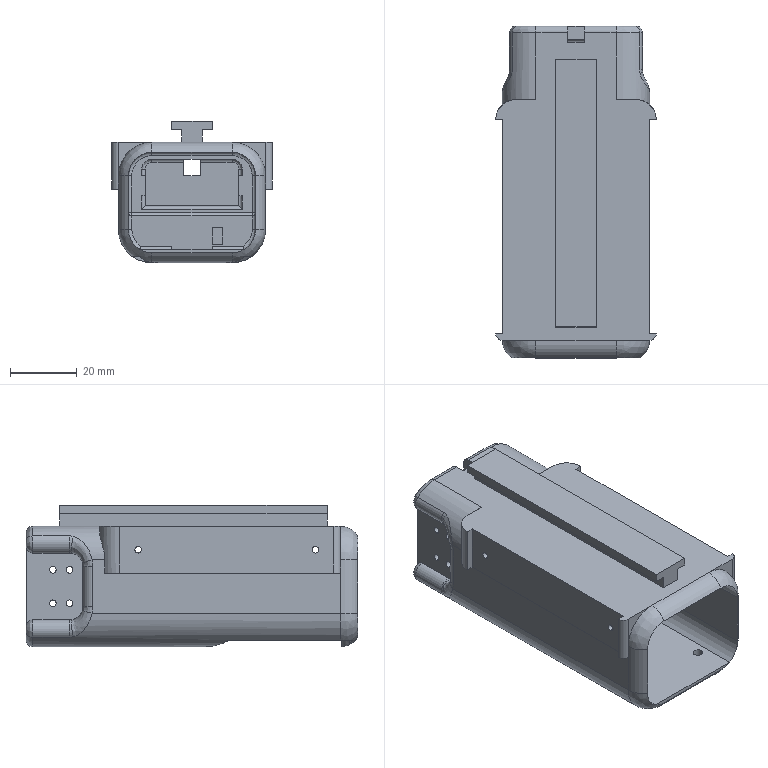Part | SolidWorks | features BaseBody 1 | 1 solid | 213 faces | box 48 x 99.2 x 42.3 mm | volume 57189 mm3 | plane 91 | cylinder 90 | spline 32 | commonest cylinder face diameters 2 x49 6 x8 2.9 x6 12 x6 14 x6 4 x5